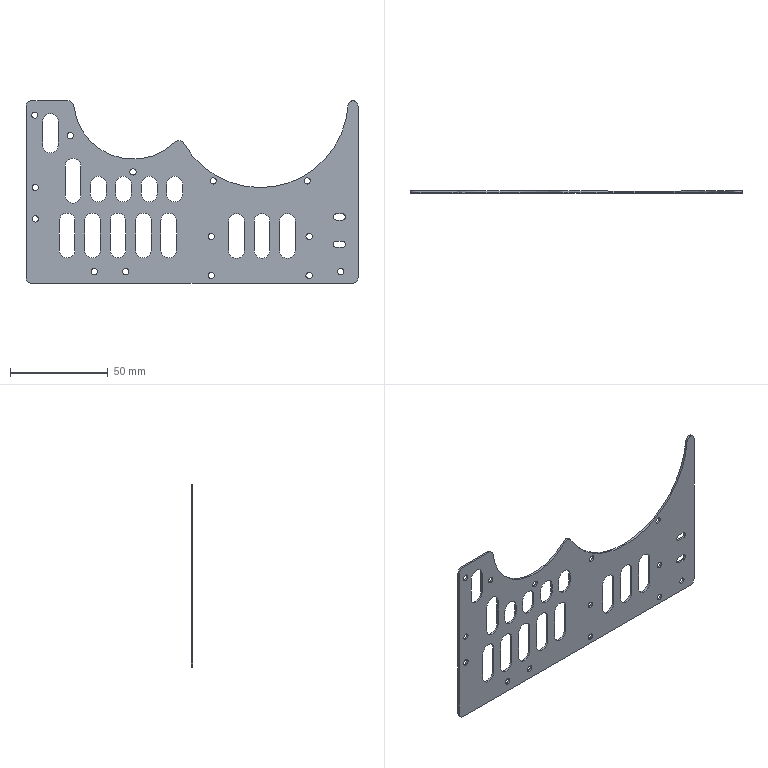Part | SolidWorks | features ICE 12, Fillet 3, Extrusion 1 | 1 solid | 125 faces | box 169.72 x 1 x 93.5 mm | volume 9219 mm3 | cylinder 87 | plane 38 | commonest cylinder face diameters 3.2 x32 8 x30 8.117 x12 6 x8 4 x2 90 x2